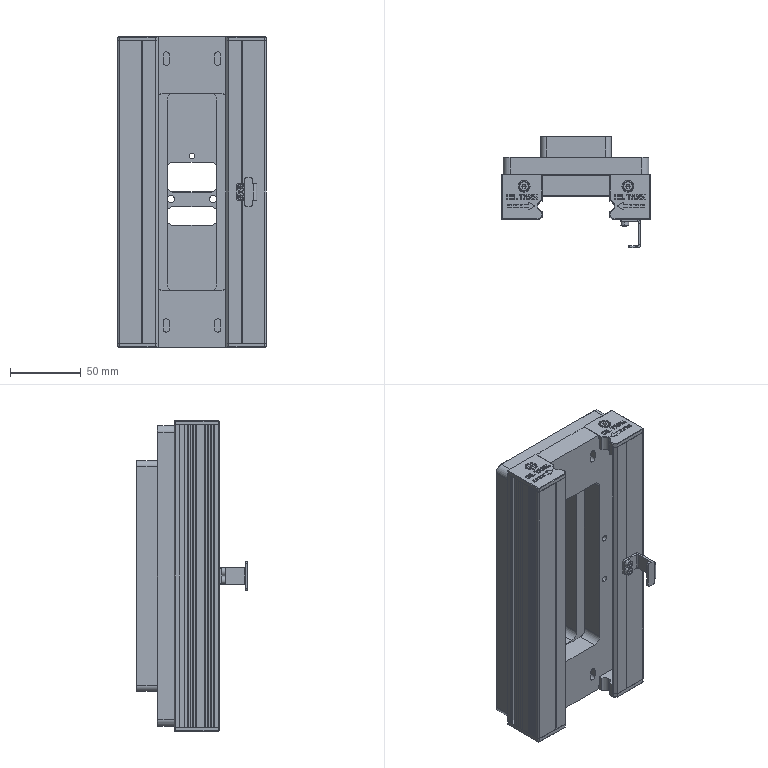Part | SolidWorks | features BaseBody 33 | 33 solids | 1926 faces | box 105 x 79 x 220 mm | volume 575496 mm3 | plane 1132 | cylinder 522 | cone 192 | torus 48 | spline 32 | commonest cylinder face diameters 0.4 x92 0.2 x90 8 x40 5 x38 10 x28 4.2 x26